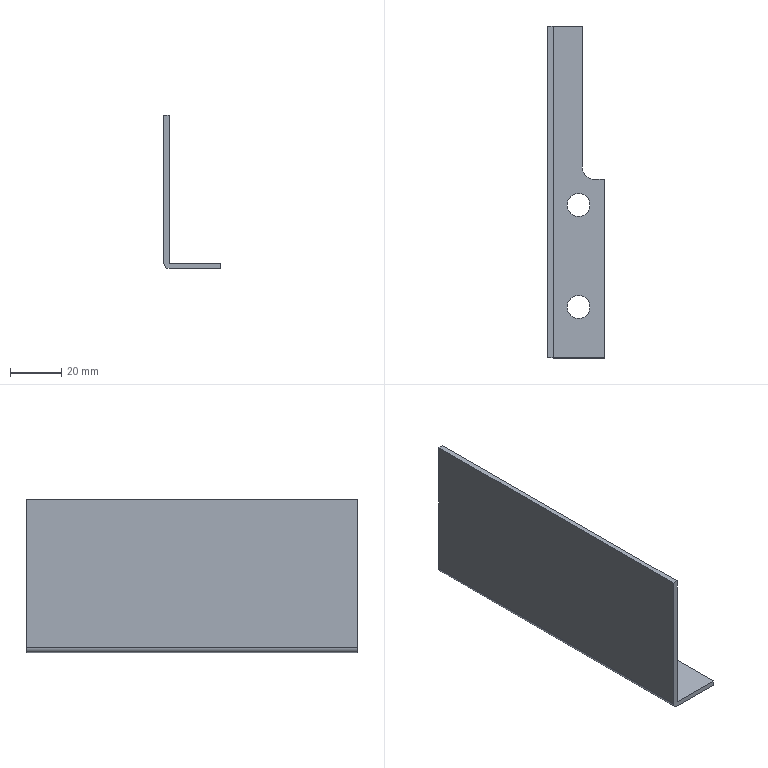Part | STEP file | lll_id4906_x_t | 1 solid | 14 faces | box 22 x 130 x 60 mm | volume 19414 mm3 | plane 10 | cylinder 4 | commonest cylinder face diameters 9 x2 4 x1 10 x1
STEP:
#1=CARTESIAN_POINT('',(2530.,-280.246,-80.));
#2=VERTEX_POINT('',#1);
#3=CARTESIAN_POINT('',(2530.,-335.246,-80.));
#4=VERTEX_POINT('',#3);
#5=CARTESIAN_POINT('',(2530.,-342.246,-80.));
#6=DIRECTION('',(0.,-1.,0.));
#7=VECTOR('',#6,1.);
#8=LINE('',#5,#7);
#9=EDGE_CURVE('',#2,#4,#8,.T.);
#10=ORIENTED_EDGE('',*,*,#9,.F.);
#11=CARTESIAN_POINT('',(2530.,-280.246,-78.));
#12=VERTEX_POINT('',#11);
#13=CARTESIAN_POINT('',(2530.,-280.246,-80.));
#14=DIRECTION('',(0.,0.,1.));
#15=VECTOR('',#14,1.);
#16=LINE('',#13,#15);
#17=EDGE_CURVE('',#2,#12,#16,.T.);
#18=ORIENTED_EDGE('',*,*,#17,.T.);
#19=CARTESIAN_POINT('',(2530.,-335.246,-78.));
#20=VERTEX_POINT('',#19);
#21=CARTESIAN_POINT('',(2530.,-342.246,-78.));
#22=DIRECTION('',(0.,1.,0.));
#23=VECTOR('',#22,1.);
#24=LINE('',#21,#23);
#25=EDGE_CURVE('',#20,#12,#24,.T.);
#26=ORIENTED_EDGE('',*,*,#25,.F.);
#27=CARTESIAN_POINT('',(2530.,-335.246,6.));
#28=DIRECTION('',(0.,0.,1.));
#29=VECTOR('',#28,1.);
#30=LINE('',#27,#29);
#31=EDGE_CURVE('',#4,#20,#30,.T.);
#32=ORIENTED_EDGE('',*,*,#31,.F.);
#33=EDGE_LOOP('',(#10,#18,#26,#32));
#34=FACE_OUTER_BOUND('',#33,.T.);
#35=CARTESIAN_POINT('',(2530.,-246.5,6.));
#36=DIRECTION('',(-1.,0.,0.));
#37=DIRECTION('',(0.,0.,-1.));
#38=AXIS2_PLACEMENT_3D('',#35,#36,#37);
#39=PLANE('',#38);
#40=ADVANCED_FACE('',(#34),#39,.F.);
#41=CARTESIAN_POINT('',(2538.588,-410.246,-78.));
#42=VERTEX_POINT('',#41);
#43=CARTESIAN_POINT('',(2518.588,-410.246,-78.));
#44=VERTEX_POINT('',#43);
#45=CARTESIAN_POINT('',(2516.588,-410.246,-78.));
#46=DIRECTION('',(-1.,0.,0.));
#47=VECTOR('',#46,1.);
#48=LINE('',#45,#47);
#49=EDGE_CURVE('',#42,#44,#48,.T.);
#50=ORIENTED_EDGE('',*,*,#49,.T.);
#51=CARTESIAN_POINT('',(2518.588,-410.246,-20.));
#52=VERTEX_POINT('',#51);
#53=CARTESIAN_POINT('',(2518.588,-410.246,-10.));
#54=DIRECTION('',(0.,0.,1.));
#55=VECTOR('',#54,1.);
#56=LINE('',#53,#55);
#57=EDGE_CURVE('',#44,#52,#56,.T.);
#58=ORIENTED_EDGE('',*,*,#57,.T.);
#59=CARTESIAN_POINT('',(2516.588,-410.246,-20.));
#60=VERTEX_POINT('',#59);
#61=CARTESIAN_POINT('',(2516.588,-410.246,-20.));
#62=DIRECTION('',(1.,0.,0.));
#63=VECTOR('',#62,1.);
#64=LINE('',#61,#63);
#65=EDGE_CURVE('',#60,#52,#64,.T.);
#66=ORIENTED_EDGE('',*,*,#65,.F.);
#67=CARTESIAN_POINT('',(2516.588,-410.246,-78.));
#68=VERTEX_POINT('',#67);
#69=CARTESIAN_POINT('',(2516.588,-410.246,-10.));
#70=DIRECTION('',(0.,0.,1.));
#71=VECTOR('',#70,1.);
#72=LINE('',#69,#71);
#73=EDGE_CURVE('',#68,#60,#72,.T.);
#74=ORIENTED_EDGE('',*,*,#73,.F.);
#75=CARTESIAN_POINT('',(2518.588,-410.246,-80.));
#76=VERTEX_POINT('',#75);
#77=CARTESIAN_POINT('',(2518.588,-410.246,-78.));
#78=DIRECTION('',(0.,1.,0.));
#79=DIRECTION('',(0.,0.,1.));
#80=AXIS2_PLACEMENT_3D('',#77,#78,#79);
#81=CIRCLE('',#80,2.);
#82=EDGE_CURVE('',#76,#68,#81,.T.);
#83=ORIENTED_EDGE('',*,*,#82,.F.);
#84=CARTESIAN_POINT('',(2538.588,-410.246,-80.));
#85=VERTEX_POINT('',#84);
#86=CARTESIAN_POINT('',(2516.588,-410.246,-80.));
#87=DIRECTION('',(-1.,0.,0.));
#88=VECTOR('',#87,1.);
#89=LINE('',#86,#88);
#90=EDGE_CURVE('',#85,#76,#89,.T.);
#91=ORIENTED_EDGE('',*,*,#90,.F.);
#92=CARTESIAN_POINT('',(2538.588,-410.246,-80.));
#93=DIRECTION('',(0.,0.,1.));
#94=VECTOR('',#93,1.);
#95=LINE('',#92,#94);
#96=EDGE_CURVE('',#85,#42,#95,.T.);
#97=ORIENTED_EDGE('',*,*,#96,.T.);
#98=EDGE_LOOP('',(#50,#58,#66,#74,#83,#91,#97));
#99=FACE_OUTER_BOUND('',#98,.T.);
#100=CARTESIAN_POINT('',(2516.588,-410.246,-10.));
#101=DIRECTION('',(0.,1.,0.));
#102=DIRECTION('',(0.,0.,-1.));
#103=AXIS2_PLACEMENT_3D('',#100,#101,#102);
#104=PLANE('',#103);
#105=ADVANCED_FACE('',(#99),#104,.F.);
#106=CARTESIAN_POINT('',(2516.588,-280.246,-20.));
#107=VERTEX_POINT('',#106);
#108=CARTESIAN_POINT('',(2518.588,-280.246,-20.));
#109=VERTEX_POINT('',#108);
#110=CARTESIAN_POINT('',(2516.588,-280.246,-20.));
#111=DIRECTION('',(1.,0.,0.));
#112=VECTOR('',#111,1.);
#113=LINE('',#110,#112);
#114=EDGE_CURVE('',#107,#109,#113,.T.);
#115=ORIENTED_EDGE('',*,*,#114,.F.);
#116=CARTESIAN_POINT('',(2516.588,-342.246,-20.));
#117=DIRECTION('',(0.,1.,0.));
#118=VECTOR('',#117,1.);
#119=LINE('',#116,#118);
#120=EDGE_CURVE('',#60,#107,#119,.T.);
#121=ORIENTED_EDGE('',*,*,#120,.F.);
#122=ORIENTED_EDGE('',*,*,#65,.T.);
#123=CARTESIAN_POINT('',(2518.588,-342.246,-20.));
#124=DIRECTION('',(0.,1.,0.));
#125=VECTOR('',#124,1.);
#126=LINE('',#123,#125);
#127=EDGE_CURVE('',#52,#109,#126,.T.);
#128=ORIENTED_EDGE('',*,*,#127,.T.);
#129=EDGE_LOOP('',(#115,#121,#122,#128));
#130=FACE_OUTER_BOUND('',#129,.T.);
#131=CARTESIAN_POINT('',(2516.588,-342.246,-20.));
#132=DIRECTION('',(0.,0.,-1.));
#133=DIRECTION('',(0.,-1.,0.));
#134=AXIS2_PLACEMENT_3D('',#131,#132,#133);
#135=PLANE('',#134);
#136=ADVANCED_FACE('',(#130),#135,.F.);
#137=ORIENTED_EDGE('',*,*,#127,.F.);
#138=ORIENTED_EDGE('',*,*,#57,.F.);
#139=CARTESIAN_POINT('',(2518.588,-280.246,-78.));
#140=VERTEX_POINT('',#139);
#141=CARTESIAN_POINT('',(2518.588,-342.246,-78.));
#142=DIRECTION('',(0.,-1.,0.));
#143=VECTOR('',#142,1.);
#144=LINE('',#141,#143);
#145=EDGE_CURVE('',#140,#44,#144,.T.);
#146=ORIENTED_EDGE('',*,*,#145,.F.);
#147=CARTESIAN_POINT('',(2518.588,-280.246,-10.));
#148=DIRECTION('',(0.,0.,-1.));
#149=VECTOR('',#148,1.);
#150=LINE('',#147,#149);
#151=EDGE_CURVE('',#109,#140,#150,.T.);
#152=ORIENTED_EDGE('',*,*,#151,.F.);
#153=EDGE_LOOP('',(#137,#138,#146,#152));
#154=FACE_OUTER_BOUND('',#153,.T.);
#155=CARTESIAN_POINT('',(2518.588,-342.246,-10.));
#156=DIRECTION('',(1.,0.,0.));
#157=DIRECTION('',(0.,0.,-1.));
#158=AXIS2_PLACEMENT_3D('',#155,#156,#157);
#159=PLANE('',#158);
#160=ADVANCED_FACE('',(#154),#159,.T.);
#161=CARTESIAN_POINT('',(2528.588,-394.746,-78.));
#162=VERTEX_POINT('',#161);
#163=CARTESIAN_POINT('',(2528.588,-390.246,-78.));
#164=DIRECTION('',(0.,0.,-1.));
#165=DIRECTION('',(0.,-1.,0.));
#166=AXIS2_PLACEMENT_3D('',#163,#164,#165);
#167=CIRCLE('',#166,4.5);
#168=EDGE_CURVE('',#162,#162,#167,.T.);
#169=ORIENTED_EDGE('',*,*,#168,.T.);
#170=EDGE_LOOP('',(#169));
#171=FACE_BOUND('',#170,.T.);
#172=ORIENTED_EDGE('',*,*,#25,.T.);
#173=CARTESIAN_POINT('',(2516.588,-280.246,-78.));
#174=DIRECTION('',(1.,0.,0.));
#175=VECTOR('',#174,1.);
#176=LINE('',#173,#175);
#177=EDGE_CURVE('',#140,#12,#176,.T.);
#178=ORIENTED_EDGE('',*,*,#177,.F.);
#179=ORIENTED_EDGE('',*,*,#145,.T.);
#180=ORIENTED_EDGE('',*,*,#49,.F.);
#181=CARTESIAN_POINT('',(2538.588,-340.246,-78.));
#182=VERTEX_POINT('',#181);
#183=CARTESIAN_POINT('',(2538.588,-342.246,-78.));
#184=DIRECTION('',(0.,-1.,0.));
#185=VECTOR('',#184,1.);
#186=LINE('',#183,#185);
#187=EDGE_CURVE('',#182,#42,#186,.T.);
#188=ORIENTED_EDGE('',*,*,#187,.F.);
#189=CARTESIAN_POINT('',(2535.,-340.246,-78.));
#190=VERTEX_POINT('',#189);
#191=CARTESIAN_POINT('',(2516.588,-340.246,-78.));
#192=DIRECTION('',(1.,0.,0.));
#193=VECTOR('',#192,1.);
#194=LINE('',#191,#193);
#195=EDGE_CURVE('',#190,#182,#194,.T.);
#196=ORIENTED_EDGE('',*,*,#195,.F.);
#197=CARTESIAN_POINT('',(2535.,-335.246,-78.));
#198=DIRECTION('',(0.,0.,1.));
#199=DIRECTION('',(-1.,0.,0.));
#200=AXIS2_PLACEMENT_3D('',#197,#198,#199);
#201=CIRCLE('',#200,5.);
#202=EDGE_CURVE('',#20,#190,#201,.T.);
#203=ORIENTED_EDGE('',*,*,#202,.F.);
#204=EDGE_LOOP('',(#172,#178,#179,#180,#188,#196,#203));
#205=FACE_BOUND('',#204,.T.);
#206=CARTESIAN_POINT('',(2528.588,-354.746,-78.));
#207=VERTEX_POINT('',#206);
#208=CARTESIAN_POINT('',(2528.588,-350.246,-78.));
#209=DIRECTION('',(0.,0.,-1.));
#210=DIRECTION('',(0.,-1.,0.));
#211=AXIS2_PLACEMENT_3D('',#208,#209,#210);
#212=CIRCLE('',#211,4.5);
#213=EDGE_CURVE('',#207,#207,#212,.T.);
#214=ORIENTED_EDGE('',*,*,#213,.T.);
#215=EDGE_LOOP('',(#214));
#216=FACE_BOUND('',#215,.T.);
#217=CARTESIAN_POINT('',(2516.588,-342.246,-78.));
#218=DIRECTION('',(0.,0.,1.));
#219=DIRECTION('',(0.,-1.,0.));
#220=AXIS2_PLACEMENT_3D('',#217,#218,#219);
#221=PLANE('',#220);
#222=ADVANCED_FACE('',(#171,#205,#216),#221,.T.);
#223=CARTESIAN_POINT('',(2516.588,-280.246,-78.));
#224=VERTEX_POINT('',#223);
#225=CARTESIAN_POINT('',(2516.588,-342.246,-78.));
#226=DIRECTION('',(0.,1.,0.));
#227=VECTOR('',#226,1.);
#228=LINE('',#225,#227);
#229=EDGE_CURVE('',#68,#224,#228,.T.);
#230=ORIENTED_EDGE('',*,*,#229,.F.);
#231=ORIENTED_EDGE('',*,*,#73,.T.);
#232=ORIENTED_EDGE('',*,*,#120,.T.);
#233=CARTESIAN_POINT('',(2516.588,-280.246,-10.));
#234=DIRECTION('',(0.,0.,-1.));
#235=VECTOR('',#234,1.);
#236=LINE('',#233,#235);
#237=EDGE_CURVE('',#107,#224,#236,.T.);
#238=ORIENTED_EDGE('',*,*,#237,.T.);
#239=EDGE_LOOP('',(#230,#231,#232,#238));
#240=FACE_OUTER_BOUND('',#239,.T.);
#241=CARTESIAN_POINT('',(2516.588,-342.246,-10.));
#242=DIRECTION('',(1.,0.,0.));
#243=DIRECTION('',(0.,0.,-1.));
#244=AXIS2_PLACEMENT_3D('',#241,#242,#243);
#245=PLANE('',#244);
#246=ADVANCED_FACE('',(#240),#245,.F.);
#247=ORIENTED_EDGE('',*,*,#90,.T.);
#248=CARTESIAN_POINT('',(2518.588,-280.246,-80.));
#249=VERTEX_POINT('',#248);
#250=CARTESIAN_POINT('',(2518.588,-342.246,-80.));
#251=DIRECTION('',(0.,-1.,0.));
#252=VECTOR('',#251,1.);
#253=LINE('',#250,#252);
#254=EDGE_CURVE('',#249,#76,#253,.T.);
#255=ORIENTED_EDGE('',*,*,#254,.F.);
#256=CARTESIAN_POINT('',(2516.588,-280.246,-80.));
#257=DIRECTION('',(1.,0.,0.));
#258=VECTOR('',#257,1.);
#259=LINE('',#256,#258);
#260=EDGE_CURVE('',#249,#2,#259,.T.);
#261=ORIENTED_EDGE('',*,*,#260,.T.);
#262=ORIENTED_EDGE('',*,*,#9,.T.);
#263=CARTESIAN_POINT('',(2535.,-340.246,-80.));
#264=VERTEX_POINT('',#263);
#265=CARTESIAN_POINT('',(2535.,-335.246,-80.));
#266=DIRECTION('',(0.,0.,-1.));
#267=DIRECTION('',(-1.,0.,0.));
#268=AXIS2_PLACEMENT_3D('',#265,#266,#267);
#269=CIRCLE('',#268,5.);
#270=EDGE_CURVE('',#264,#4,#269,.T.);
#271=ORIENTED_EDGE('',*,*,#270,.F.);
#272=CARTESIAN_POINT('',(2538.588,-340.246,-80.));
#273=VERTEX_POINT('',#272);
#274=CARTESIAN_POINT('',(2516.588,-340.246,-80.));
#275=DIRECTION('',(1.,0.,0.));
#276=VECTOR('',#275,1.);
#277=LINE('',#274,#276);
#278=EDGE_CURVE('',#264,#273,#277,.T.);
#279=ORIENTED_EDGE('',*,*,#278,.T.);
#280=CARTESIAN_POINT('',(2538.588,-342.246,-80.));
#281=DIRECTION('',(0.,-1.,0.));
#282=VECTOR('',#281,1.);
#283=LINE('',#280,#282);
#284=EDGE_CURVE('',#273,#85,#283,.T.);
#285=ORIENTED_EDGE('',*,*,#284,.T.);
#286=EDGE_LOOP('',(#247,#255,#261,#262,#271,#279,#285));
#287=FACE_BOUND('',#286,.T.);
#288=CARTESIAN_POINT('',(2528.588,-394.746,-80.));
#289=VERTEX_POINT('',#288);
#290=CARTESIAN_POINT('',(2528.588,-390.246,-80.));
#291=DIRECTION('',(0.,0.,-1.));
#292=DIRECTION('',(0.,-1.,0.));
#293=AXIS2_PLACEMENT_3D('',#290,#291,#292);
#294=CIRCLE('',#293,4.5);
#295=EDGE_CURVE('',#289,#289,#294,.T.);
#296=ORIENTED_EDGE('',*,*,#295,.F.);
#297=EDGE_LOOP('',(#296));
#298=FACE_BOUND('',#297,.T.);
#299=CARTESIAN_POINT('',(2528.588,-354.746,-80.));
#300=VERTEX_POINT('',#299);
#301=CARTESIAN_POINT('',(2528.588,-350.246,-80.));
#302=DIRECTION('',(0.,0.,-1.));
#303=DIRECTION('',(0.,-1.,0.));
#304=AXIS2_PLACEMENT_3D('',#301,#302,#303);
#305=CIRCLE('',#304,4.5);
#306=EDGE_CURVE('',#300,#300,#305,.T.);
#307=ORIENTED_EDGE('',*,*,#306,.F.);
#308=EDGE_LOOP('',(#307));
#309=FACE_BOUND('',#308,.T.);
#310=CARTESIAN_POINT('',(2516.588,-342.246,-80.));
#311=DIRECTION('',(0.,0.,1.));
#312=DIRECTION('',(0.,-1.,0.));
#313=AXIS2_PLACEMENT_3D('',#310,#311,#312);
#314=PLANE('',#313);
#315=ADVANCED_FACE('',(#287,#298,#309),#314,.F.);
#316=ORIENTED_EDGE('',*,*,#82,.T.);
#317=ORIENTED_EDGE('',*,*,#229,.T.);
#318=CARTESIAN_POINT('',(2518.588,-280.246,-78.));
#319=DIRECTION('',(0.,-1.,0.));
#320=DIRECTION('',(0.,0.,1.));
#321=AXIS2_PLACEMENT_3D('',#318,#319,#320);
#322=CIRCLE('',#321,2.);
#323=EDGE_CURVE('',#224,#249,#322,.T.);
#324=ORIENTED_EDGE('',*,*,#323,.T.);
#325=ORIENTED_EDGE('',*,*,#254,.T.);
#326=EDGE_LOOP('',(#316,#317,#324,#325));
#327=FACE_OUTER_BOUND('',#326,.T.);
#328=CARTESIAN_POINT('',(2518.588,-342.246,-78.));
#329=DIRECTION('',(0.,-1.,0.));
#330=DIRECTION('',(0.,0.,-1.));
#331=AXIS2_PLACEMENT_3D('',#328,#329,#330);
#332=CYLINDRICAL_SURFACE('',#331,2.);
#333=ADVANCED_FACE('',(#327),#332,.T.);
#334=ORIENTED_EDGE('',*,*,#295,.T.);
#335=EDGE_LOOP('',(#334));
#336=FACE_BOUND('',#335,.T.);
#337=ORIENTED_EDGE('',*,*,#168,.F.);
#338=EDGE_LOOP('',(#337));
#339=FACE_BOUND('',#338,.T.);
#340=CARTESIAN_POINT('',(2528.588,-390.246,-58.));
#341=DIRECTION('',(0.,0.,-1.));
#342=DIRECTION('',(0.,1.,0.));
#343=AXIS2_PLACEMENT_3D('',#340,#341,#342);
#344=CYLINDRICAL_SURFACE('',#343,4.5);
#345=ADVANCED_FACE('',(#336,#339),#344,.F.);
#346=ORIENTED_EDGE('',*,*,#17,.F.);
#347=ORIENTED_EDGE('',*,*,#260,.F.);
#348=ORIENTED_EDGE('',*,*,#323,.F.);
#349=ORIENTED_EDGE('',*,*,#237,.F.);
#350=ORIENTED_EDGE('',*,*,#114,.T.);
#351=ORIENTED_EDGE('',*,*,#151,.T.);
#352=ORIENTED_EDGE('',*,*,#177,.T.);
#353=EDGE_LOOP('',(#346,#347,#348,#349,#350,#351,#352));
#354=FACE_OUTER_BOUND('',#353,.T.);
#355=CARTESIAN_POINT('',(2516.588,-280.246,-80.));
#356=DIRECTION('',(0.,1.,0.));
#357=DIRECTION('',(1.,0.,0.));
#358=AXIS2_PLACEMENT_3D('',#355,#356,#357);
#359=PLANE('',#358);
#360=ADVANCED_FACE('',(#354),#359,.T.);
#361=ORIENTED_EDGE('',*,*,#306,.T.);
#362=EDGE_LOOP('',(#361));
#363=FACE_BOUND('',#362,.T.);
#364=ORIENTED_EDGE('',*,*,#213,.F.);
#365=EDGE_LOOP('',(#364));
#366=FACE_BOUND('',#365,.T.);
#367=CARTESIAN_POINT('',(2528.588,-350.246,-58.));
#368=DIRECTION('',(0.,0.,-1.));
#369=DIRECTION('',(0.,1.,0.));
#370=AXIS2_PLACEMENT_3D('',#367,#368,#369);
#371=CYLINDRICAL_SURFACE('',#370,4.5);
#372=ADVANCED_FACE('',(#363,#366),#371,.F.);
#373=ORIENTED_EDGE('',*,*,#96,.F.);
#374=ORIENTED_EDGE('',*,*,#284,.F.);
#375=CARTESIAN_POINT('',(2538.588,-340.246,-80.));
#376=DIRECTION('',(0.,0.,1.));
#377=VECTOR('',#376,1.);
#378=LINE('',#375,#377);
#379=EDGE_CURVE('',#273,#182,#378,.T.);
#380=ORIENTED_EDGE('',*,*,#379,.T.);
#381=ORIENTED_EDGE('',*,*,#187,.T.);
#382=EDGE_LOOP('',(#373,#374,#380,#381));
#383=FACE_OUTER_BOUND('',#382,.T.);
#384=CARTESIAN_POINT('',(2538.588,-342.246,-80.));
#385=DIRECTION('',(1.,0.,0.));
#386=DIRECTION('',(0.,-1.,0.));
#387=AXIS2_PLACEMENT_3D('',#384,#385,#386);
#388=PLANE('',#387);
#389=ADVANCED_FACE('',(#383),#388,.T.);
#390=ORIENTED_EDGE('',*,*,#195,.T.);
#391=ORIENTED_EDGE('',*,*,#379,.F.);
#392=ORIENTED_EDGE('',*,*,#278,.F.);
#393=CARTESIAN_POINT('',(2535.,-340.246,-80.));
#394=DIRECTION('',(0.,0.,-1.));
#395=VECTOR('',#394,1.);
#396=LINE('',#393,#395);
#397=EDGE_CURVE('',#190,#264,#396,.T.);
#398=ORIENTED_EDGE('',*,*,#397,.F.);
#399=EDGE_LOOP('',(#390,#391,#392,#398));
#400=FACE_OUTER_BOUND('',#399,.T.);
#401=CARTESIAN_POINT('',(2516.588,-340.246,-80.));
#402=DIRECTION('',(0.,1.,0.));
#403=DIRECTION('',(1.,0.,0.));
#404=AXIS2_PLACEMENT_3D('',#401,#402,#403);
#405=PLANE('',#404);
#406=ADVANCED_FACE('',(#400),#405,.T.);
#407=ORIENTED_EDGE('',*,*,#202,.T.);
#408=ORIENTED_EDGE('',*,*,#397,.T.);
#409=ORIENTED_EDGE('',*,*,#270,.T.);
#410=ORIENTED_EDGE('',*,*,#31,.T.);
#411=EDGE_LOOP('',(#407,#408,#409,#410));
#412=FACE_OUTER_BOUND('',#411,.T.);
#413=CARTESIAN_POINT('',(2535.,-335.246,-80.));
#414=DIRECTION('',(0.,0.,-1.));
#415=DIRECTION('',(1.,0.,0.));
#416=AXIS2_PLACEMENT_3D('',#413,#414,#415);
#417=CYLINDRICAL_SURFACE('',#416,5.);
#418=ADVANCED_FACE('',(#412),#417,.F.);
#419=CLOSED_SHELL('',(#40,#105,#136,#160,#222,#246,#315,#333,#345,#360,#372,#389,#406,#418));
#420=MANIFOLD_SOLID_BREP('',#419);
#421=(LENGTH_UNIT()NAMED_UNIT(*)SI_UNIT(.MILLI.,.METRE.));
#422=UNCERTAINTY_MEASURE_WITH_UNIT(LENGTH_MEASURE(0.00002),#421,'','');
#423=(NAMED_UNIT(*)PLANE_ANGLE_UNIT()SI_UNIT($,.RADIAN.));
#424=PLANE_ANGLE_MEASURE_WITH_UNIT(PLANE_ANGLE_MEASURE(0.01745),#423);
#425=DIMENSIONAL_EXPONENTS(0.,0.,0.,0.,0.,0.,0.);
#426=(CONVERSION_BASED_UNIT('DEGREE',#424)NAMED_UNIT(#425)PLANE_ANGLE_UNIT());
#427=(NAMED_UNIT(*)SI_UNIT($,.STERADIAN.)SOLID_ANGLE_UNIT());
#428=(GEOMETRIC_REPRESENTATION_CONTEXT(3)GLOBAL_UNCERTAINTY_ASSIGNED_CONTEXT((#422))GLOBAL_UNIT_ASSIGNED_CONTEXT((#421,#426,#427))REPRESENTATION_CONTEXT('',''));
#429=ADVANCED_BREP_SHAPE_REPRESENTATION('',(#420),#428);